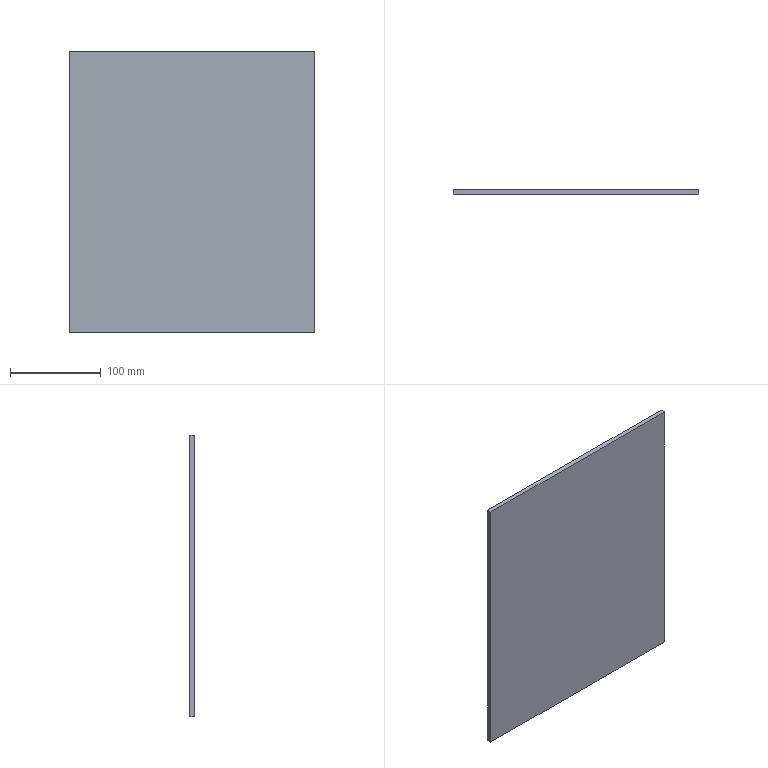Part | SolidWorks | features Extrusion 1 | 1 solid | 6 faces | box 270 x 5 x 310 mm | volume 418500 mm3 | plane 6
STEP:
#1=CARTESIAN_POINT('',(135.,0.,155.));
#2=VERTEX_POINT('',#1);
#3=CARTESIAN_POINT('',(135.,0.,-155.));
#4=VERTEX_POINT('',#3);
#5=CARTESIAN_POINT('',(135.,0.,-155.));
#6=DIRECTION('',(0.,0.,-1.));
#7=VECTOR('',#6,1000.);
#8=LINE('',#5,#7);
#9=EDGE_CURVE('',#2,#4,#8,.T.);
#10=ORIENTED_EDGE('',*,*,#9,.T.);
#11=CARTESIAN_POINT('',(135.,5.,-155.));
#12=VERTEX_POINT('',#11);
#13=CARTESIAN_POINT('',(135.,5.,-155.));
#14=DIRECTION('',(0.,-1.,0.));
#15=VECTOR('',#14,1000.);
#16=LINE('',#13,#15);
#17=EDGE_CURVE('',#12,#4,#16,.T.);
#18=ORIENTED_EDGE('',*,*,#17,.F.);
#19=CARTESIAN_POINT('',(135.,5.,155.));
#20=VERTEX_POINT('',#19);
#21=CARTESIAN_POINT('',(135.,5.,-155.));
#22=DIRECTION('',(0.,0.,-1.));
#23=VECTOR('',#22,1000.);
#24=LINE('',#21,#23);
#25=EDGE_CURVE('',#20,#12,#24,.T.);
#26=ORIENTED_EDGE('',*,*,#25,.F.);
#27=CARTESIAN_POINT('',(135.,5.,155.));
#28=DIRECTION('',(0.,-1.,0.));
#29=VECTOR('',#28,1000.);
#30=LINE('',#27,#29);
#31=EDGE_CURVE('',#20,#2,#30,.T.);
#32=ORIENTED_EDGE('',*,*,#31,.T.);
#33=EDGE_LOOP('',(#10,#18,#26,#32));
#34=FACE_OUTER_BOUND('',#33,.T.);
#35=CARTESIAN_POINT('',(135.,5.,-155.));
#36=DIRECTION('',(-1.,0.,0.));
#37=DIRECTION('',(0.,0.,1.));
#38=AXIS2_PLACEMENT_3D('',#35,#36,#37);
#39=PLANE('',#38);
#40=ADVANCED_FACE('',(#34),#39,.F.);
#41=CARTESIAN_POINT('',(-135.,0.,-155.));
#42=VERTEX_POINT('',#41);
#43=CARTESIAN_POINT('',(-135.,0.,-155.));
#44=DIRECTION('',(-1.,0.,0.));
#45=VECTOR('',#44,1000.);
#46=LINE('',#43,#45);
#47=EDGE_CURVE('',#4,#42,#46,.T.);
#48=ORIENTED_EDGE('',*,*,#47,.T.);
#49=CARTESIAN_POINT('',(-135.,5.,-155.));
#50=VERTEX_POINT('',#49);
#51=CARTESIAN_POINT('',(-135.,5.,-155.));
#52=DIRECTION('',(0.,-1.,0.));
#53=VECTOR('',#52,1000.);
#54=LINE('',#51,#53);
#55=EDGE_CURVE('',#50,#42,#54,.T.);
#56=ORIENTED_EDGE('',*,*,#55,.F.);
#57=CARTESIAN_POINT('',(-135.,5.,-155.));
#58=DIRECTION('',(-1.,0.,0.));
#59=VECTOR('',#58,1000.);
#60=LINE('',#57,#59);
#61=EDGE_CURVE('',#12,#50,#60,.T.);
#62=ORIENTED_EDGE('',*,*,#61,.F.);
#63=ORIENTED_EDGE('',*,*,#17,.T.);
#64=EDGE_LOOP('',(#48,#56,#62,#63));
#65=FACE_OUTER_BOUND('',#64,.T.);
#66=CARTESIAN_POINT('',(-135.,5.,-155.));
#67=DIRECTION('',(0.,0.,1.));
#68=DIRECTION('',(1.,0.,0.));
#69=AXIS2_PLACEMENT_3D('',#66,#67,#68);
#70=PLANE('',#69);
#71=ADVANCED_FACE('',(#65),#70,.F.);
#72=CARTESIAN_POINT('',(-135.,0.,155.));
#73=VERTEX_POINT('',#72);
#74=CARTESIAN_POINT('',(-135.,0.,-155.));
#75=DIRECTION('',(0.,0.,1.));
#76=VECTOR('',#75,1000.);
#77=LINE('',#74,#76);
#78=EDGE_CURVE('',#42,#73,#77,.T.);
#79=ORIENTED_EDGE('',*,*,#78,.T.);
#80=CARTESIAN_POINT('',(-135.,5.,155.));
#81=VERTEX_POINT('',#80);
#82=CARTESIAN_POINT('',(-135.,5.,155.));
#83=DIRECTION('',(0.,-1.,0.));
#84=VECTOR('',#83,1000.);
#85=LINE('',#82,#84);
#86=EDGE_CURVE('',#81,#73,#85,.T.);
#87=ORIENTED_EDGE('',*,*,#86,.F.);
#88=CARTESIAN_POINT('',(-135.,5.,-155.));
#89=DIRECTION('',(0.,0.,1.));
#90=VECTOR('',#89,1000.);
#91=LINE('',#88,#90);
#92=EDGE_CURVE('',#50,#81,#91,.T.);
#93=ORIENTED_EDGE('',*,*,#92,.F.);
#94=ORIENTED_EDGE('',*,*,#55,.T.);
#95=EDGE_LOOP('',(#79,#87,#93,#94));
#96=FACE_OUTER_BOUND('',#95,.T.);
#97=CARTESIAN_POINT('',(-135.,5.,-155.));
#98=DIRECTION('',(1.,0.,0.));
#99=DIRECTION('',(0.,0.,-1.));
#100=AXIS2_PLACEMENT_3D('',#97,#98,#99);
#101=PLANE('',#100);
#102=ADVANCED_FACE('',(#96),#101,.F.);
#103=CARTESIAN_POINT('',(-135.,0.,155.));
#104=DIRECTION('',(1.,0.,0.));
#105=VECTOR('',#104,1000.);
#106=LINE('',#103,#105);
#107=EDGE_CURVE('',#73,#2,#106,.T.);
#108=ORIENTED_EDGE('',*,*,#107,.T.);
#109=ORIENTED_EDGE('',*,*,#31,.F.);
#110=CARTESIAN_POINT('',(-135.,5.,155.));
#111=DIRECTION('',(1.,0.,0.));
#112=VECTOR('',#111,1000.);
#113=LINE('',#110,#112);
#114=EDGE_CURVE('',#81,#20,#113,.T.);
#115=ORIENTED_EDGE('',*,*,#114,.F.);
#116=ORIENTED_EDGE('',*,*,#86,.T.);
#117=EDGE_LOOP('',(#108,#109,#115,#116));
#118=FACE_OUTER_BOUND('',#117,.T.);
#119=CARTESIAN_POINT('',(-135.,5.,155.));
#120=DIRECTION('',(0.,0.,-1.));
#121=DIRECTION('',(-1.,0.,0.));
#122=AXIS2_PLACEMENT_3D('',#119,#120,#121);
#123=PLANE('',#122);
#124=ADVANCED_FACE('',(#118),#123,.F.);
#125=ORIENTED_EDGE('',*,*,#25,.T.);
#126=ORIENTED_EDGE('',*,*,#61,.T.);
#127=ORIENTED_EDGE('',*,*,#92,.T.);
#128=ORIENTED_EDGE('',*,*,#114,.T.);
#129=EDGE_LOOP('',(#125,#126,#127,#128));
#130=FACE_OUTER_BOUND('',#129,.T.);
#131=CARTESIAN_POINT('',(0.,5.,0.));
#132=DIRECTION('',(0.,1.,0.));
#133=DIRECTION('',(0.,0.,1.));
#134=AXIS2_PLACEMENT_3D('',#131,#132,#133);
#135=PLANE('',#134);
#136=ADVANCED_FACE('',(#130),#135,.T.);
#137=ORIENTED_EDGE('',*,*,#9,.F.);
#138=ORIENTED_EDGE('',*,*,#107,.F.);
#139=ORIENTED_EDGE('',*,*,#78,.F.);
#140=ORIENTED_EDGE('',*,*,#47,.F.);
#141=EDGE_LOOP('',(#137,#138,#139,#140));
#142=FACE_OUTER_BOUND('',#141,.T.);
#143=CARTESIAN_POINT('',(0.,0.,0.));
#144=DIRECTION('',(0.,1.,0.));
#145=DIRECTION('',(0.,0.,1.));
#146=AXIS2_PLACEMENT_3D('',#143,#144,#145);
#147=PLANE('',#146);
#148=ADVANCED_FACE('',(#142),#147,.F.);
#149=CLOSED_SHELL('',(#40,#71,#102,#124,#136,#148));
#150=MANIFOLD_SOLID_BREP('',#149);
#151=CARTESIAN_POINT('',(0.,0.,0.));
#152=DIRECTION('',(0.,0.,1.));
#153=DIRECTION('',(1.,0.,0.));
#154=AXIS2_PLACEMENT_3D('',#151,#152,#153);
#155=(LENGTH_UNIT()NAMED_UNIT(*)SI_UNIT(.MILLI.,.METRE.));
#156=UNCERTAINTY_MEASURE_WITH_UNIT(LENGTH_MEASURE(0.00001),#155,'','');
#157=(NAMED_UNIT(*)PLANE_ANGLE_UNIT()SI_UNIT($,.RADIAN.));
#158=(NAMED_UNIT(*)SI_UNIT($,.STERADIAN.)SOLID_ANGLE_UNIT());
#159=(GEOMETRIC_REPRESENTATION_CONTEXT(3)GLOBAL_UNCERTAINTY_ASSIGNED_CONTEXT((#156))GLOBAL_UNIT_ASSIGNED_CONTEXT((#155,#157,#158))REPRESENTATION_CONTEXT('',''));
#160=ADVANCED_BREP_SHAPE_REPRESENTATION('',(#150,#154),#159);